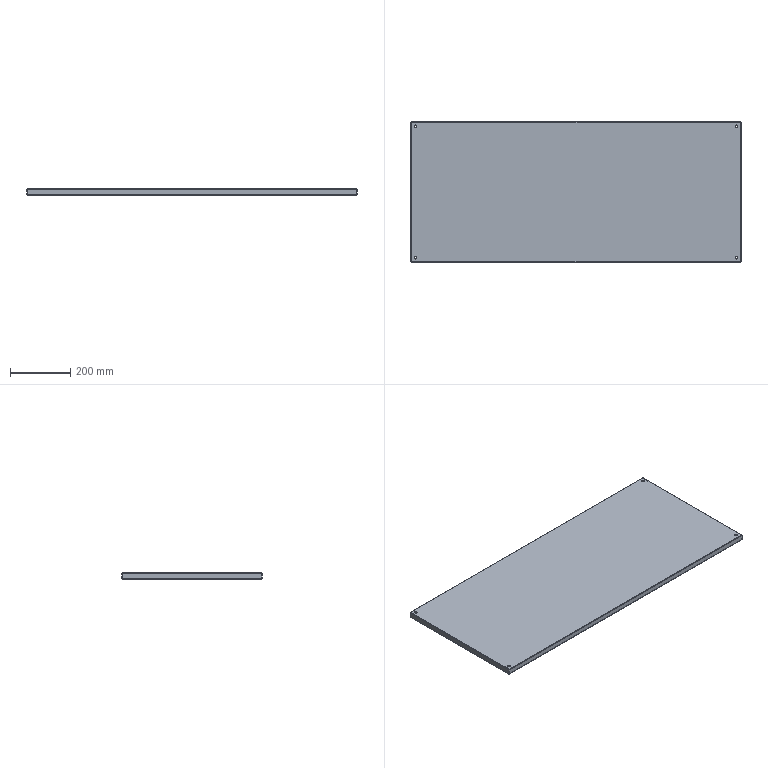Part | SolidWorks | features EdgeFlange 2, FlatPattern 1, HoleWzd 1, SMBaseFlange 1, SheetMetal 1 | 1 solid | 78 faces | box 1098 x 468 x 20 mm | volume 890194 mm3 | plane 38 | cylinder 24 | spline 16 | commonest cylinder face diameters 1.473 x8 4.473 x8 8 x8